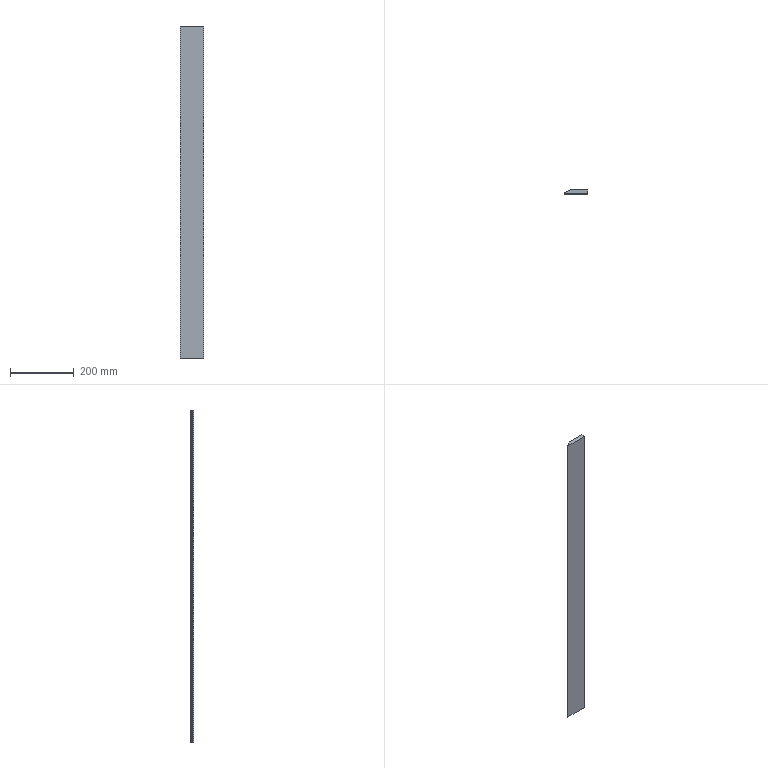Part | SolidWorks | features FlatPattern 1, SMBaseFlange 1, SheetMetal 1 | 1 solid | 7 faces | box 75 x 12 x 1040 mm | volume 832000 mm3 | plane 7
STEP:
#1=CARTESIAN_POINT('',(55.,0.,0.));
#2=VERTEX_POINT('',#1);
#3=CARTESIAN_POINT('',(55.,12.,0.));
#4=VERTEX_POINT('',#3);
#5=CARTESIAN_POINT('',(55.,12.,0.));
#6=DIRECTION('',(0.,1.,0.));
#7=VECTOR('',#6,1000.);
#8=LINE('',#5,#7);
#9=EDGE_CURVE('',#2,#4,#8,.T.);
#10=ORIENTED_EDGE('',*,*,#9,.F.);
#11=CARTESIAN_POINT('',(55.,0.,-1040.));
#12=VERTEX_POINT('',#11);
#13=CARTESIAN_POINT('',(55.,0.,-1040.));
#14=DIRECTION('',(0.,0.,1.));
#15=VECTOR('',#14,1000.);
#16=LINE('',#13,#15);
#17=EDGE_CURVE('',#12,#2,#16,.T.);
#18=ORIENTED_EDGE('',*,*,#17,.F.);
#19=CARTESIAN_POINT('',(55.,12.,-1040.));
#20=VERTEX_POINT('',#19);
#21=CARTESIAN_POINT('',(55.,12.,-1040.));
#22=DIRECTION('',(0.,1.,0.));
#23=VECTOR('',#22,1000.);
#24=LINE('',#21,#23);
#25=EDGE_CURVE('',#12,#20,#24,.T.);
#26=ORIENTED_EDGE('',*,*,#25,.T.);
#27=CARTESIAN_POINT('',(55.,12.,-1040.));
#28=DIRECTION('',(0.,0.,1.));
#29=VECTOR('',#28,1000.);
#30=LINE('',#27,#29);
#31=EDGE_CURVE('',#20,#4,#30,.T.);
#32=ORIENTED_EDGE('',*,*,#31,.T.);
#33=EDGE_LOOP('',(#10,#18,#26,#32));
#34=FACE_OUTER_BOUND('',#33,.T.);
#35=CARTESIAN_POINT('',(55.,12.,-1040.));
#36=DIRECTION('',(1.,0.,0.));
#37=DIRECTION('',(0.,1.,0.));
#38=AXIS2_PLACEMENT_3D('',#35,#36,#37);
#39=PLANE('',#38);
#40=ADVANCED_FACE('',(#34),#39,.T.);
#41=CARTESIAN_POINT('',(-20.,0.,0.));
#42=VERTEX_POINT('',#41);
#43=CARTESIAN_POINT('',(55.,0.,0.));
#44=DIRECTION('',(1.,0.,0.));
#45=VECTOR('',#44,1000.);
#46=LINE('',#43,#45);
#47=EDGE_CURVE('',#42,#2,#46,.T.);
#48=ORIENTED_EDGE('',*,*,#47,.F.);
#49=CARTESIAN_POINT('',(-20.,0.,-1040.));
#50=VERTEX_POINT('',#49);
#51=CARTESIAN_POINT('',(-20.,0.,-1040.));
#52=DIRECTION('',(0.,0.,1.));
#53=VECTOR('',#52,1000.);
#54=LINE('',#51,#53);
#55=EDGE_CURVE('',#50,#42,#54,.T.);
#56=ORIENTED_EDGE('',*,*,#55,.F.);
#57=CARTESIAN_POINT('',(55.,0.,-1040.));
#58=DIRECTION('',(1.,0.,0.));
#59=VECTOR('',#58,1000.);
#60=LINE('',#57,#59);
#61=EDGE_CURVE('',#50,#12,#60,.T.);
#62=ORIENTED_EDGE('',*,*,#61,.T.);
#63=ORIENTED_EDGE('',*,*,#17,.T.);
#64=EDGE_LOOP('',(#48,#56,#62,#63));
#65=FACE_OUTER_BOUND('',#64,.T.);
#66=CARTESIAN_POINT('',(55.,0.,-1040.));
#67=DIRECTION('',(0.,-1.,0.));
#68=DIRECTION('',(1.,0.,0.));
#69=AXIS2_PLACEMENT_3D('',#66,#67,#68);
#70=PLANE('',#69);
#71=ADVANCED_FACE('',(#65),#70,.T.);
#72=CARTESIAN_POINT('',(-20.,2.,0.));
#73=VERTEX_POINT('',#72);
#74=CARTESIAN_POINT('',(-20.,0.,0.));
#75=DIRECTION('',(0.,-1.,0.));
#76=VECTOR('',#75,1000.);
#77=LINE('',#74,#76);
#78=EDGE_CURVE('',#73,#42,#77,.T.);
#79=ORIENTED_EDGE('',*,*,#78,.F.);
#80=CARTESIAN_POINT('',(-20.,2.,-1040.));
#81=VERTEX_POINT('',#80);
#82=CARTESIAN_POINT('',(-20.,2.,-1040.));
#83=DIRECTION('',(0.,0.,1.));
#84=VECTOR('',#83,1000.);
#85=LINE('',#82,#84);
#86=EDGE_CURVE('',#81,#73,#85,.T.);
#87=ORIENTED_EDGE('',*,*,#86,.F.);
#88=CARTESIAN_POINT('',(-20.,0.,-1040.));
#89=DIRECTION('',(0.,-1.,0.));
#90=VECTOR('',#89,1000.);
#91=LINE('',#88,#90);
#92=EDGE_CURVE('',#81,#50,#91,.T.);
#93=ORIENTED_EDGE('',*,*,#92,.T.);
#94=ORIENTED_EDGE('',*,*,#55,.T.);
#95=EDGE_LOOP('',(#79,#87,#93,#94));
#96=FACE_OUTER_BOUND('',#95,.T.);
#97=CARTESIAN_POINT('',(-20.,0.,-1040.));
#98=DIRECTION('',(-1.,0.,0.));
#99=DIRECTION('',(0.,-1.,0.));
#100=AXIS2_PLACEMENT_3D('',#97,#98,#99);
#101=PLANE('',#100);
#102=ADVANCED_FACE('',(#96),#101,.T.);
#103=CARTESIAN_POINT('',(0.,12.,0.));
#104=VERTEX_POINT('',#103);
#105=CARTESIAN_POINT('',(-20.,2.,0.));
#106=DIRECTION('',(-0.8944,-0.4472,0.));
#107=VECTOR('',#106,1000.);
#108=LINE('',#105,#107);
#109=EDGE_CURVE('',#104,#73,#108,.T.);
#110=ORIENTED_EDGE('',*,*,#109,.F.);
#111=CARTESIAN_POINT('',(0.,12.,-1040.));
#112=VERTEX_POINT('',#111);
#113=CARTESIAN_POINT('',(0.,12.,-1040.));
#114=DIRECTION('',(0.,0.,1.));
#115=VECTOR('',#114,1000.);
#116=LINE('',#113,#115);
#117=EDGE_CURVE('',#112,#104,#116,.T.);
#118=ORIENTED_EDGE('',*,*,#117,.F.);
#119=CARTESIAN_POINT('',(-20.,2.,-1040.));
#120=DIRECTION('',(-0.8944,-0.4472,0.));
#121=VECTOR('',#120,1000.);
#122=LINE('',#119,#121);
#123=EDGE_CURVE('',#112,#81,#122,.T.);
#124=ORIENTED_EDGE('',*,*,#123,.T.);
#125=ORIENTED_EDGE('',*,*,#86,.T.);
#126=EDGE_LOOP('',(#110,#118,#124,#125));
#127=FACE_OUTER_BOUND('',#126,.T.);
#128=CARTESIAN_POINT('',(-20.,2.,-1040.));
#129=DIRECTION('',(-0.4472,0.8944,0.));
#130=DIRECTION('',(-0.8944,-0.4472,0.));
#131=AXIS2_PLACEMENT_3D('',#128,#129,#130);
#132=PLANE('',#131);
#133=ADVANCED_FACE('',(#127),#132,.T.);
#134=CARTESIAN_POINT('',(0.,12.,0.));
#135=DIRECTION('',(-1.,0.,0.));
#136=VECTOR('',#135,1000.);
#137=LINE('',#134,#136);
#138=EDGE_CURVE('',#4,#104,#137,.T.);
#139=ORIENTED_EDGE('',*,*,#138,.F.);
#140=ORIENTED_EDGE('',*,*,#31,.F.);
#141=CARTESIAN_POINT('',(0.,12.,-1040.));
#142=DIRECTION('',(-1.,0.,0.));
#143=VECTOR('',#142,1000.);
#144=LINE('',#141,#143);
#145=EDGE_CURVE('',#20,#112,#144,.T.);
#146=ORIENTED_EDGE('',*,*,#145,.T.);
#147=ORIENTED_EDGE('',*,*,#117,.T.);
#148=EDGE_LOOP('',(#139,#140,#146,#147));
#149=FACE_OUTER_BOUND('',#148,.T.);
#150=CARTESIAN_POINT('',(0.,12.,-1040.));
#151=DIRECTION('',(0.,1.,0.));
#152=DIRECTION('',(0.,0.,1.));
#153=AXIS2_PLACEMENT_3D('',#150,#151,#152);
#154=PLANE('',#153);
#155=ADVANCED_FACE('',(#149),#154,.T.);
#156=ORIENTED_EDGE('',*,*,#25,.F.);
#157=ORIENTED_EDGE('',*,*,#61,.F.);
#158=ORIENTED_EDGE('',*,*,#92,.F.);
#159=ORIENTED_EDGE('',*,*,#123,.F.);
#160=ORIENTED_EDGE('',*,*,#145,.F.);
#161=EDGE_LOOP('',(#156,#157,#158,#159,#160));
#162=FACE_OUTER_BOUND('',#161,.T.);
#163=CARTESIAN_POINT('',(0.,0.,-1040.));
#164=DIRECTION('',(0.,0.,-1.));
#165=DIRECTION('',(-1.,0.,0.));
#166=AXIS2_PLACEMENT_3D('',#163,#164,#165);
#167=PLANE('',#166);
#168=ADVANCED_FACE('',(#162),#167,.T.);
#169=ORIENTED_EDGE('',*,*,#9,.T.);
#170=ORIENTED_EDGE('',*,*,#138,.T.);
#171=ORIENTED_EDGE('',*,*,#109,.T.);
#172=ORIENTED_EDGE('',*,*,#78,.T.);
#173=ORIENTED_EDGE('',*,*,#47,.T.);
#174=EDGE_LOOP('',(#169,#170,#171,#172,#173));
#175=FACE_OUTER_BOUND('',#174,.T.);
#176=CARTESIAN_POINT('',(0.,0.,0.));
#177=DIRECTION('',(0.,0.,-1.));
#178=DIRECTION('',(-1.,0.,0.));
#179=AXIS2_PLACEMENT_3D('',#176,#177,#178);
#180=PLANE('',#179);
#181=ADVANCED_FACE('',(#175),#180,.F.);
#182=CLOSED_SHELL('',(#40,#71,#102,#133,#155,#168,#181));
#183=MANIFOLD_SOLID_BREP('',#182);
#184=CARTESIAN_POINT('',(0.,0.,0.));
#185=DIRECTION('',(0.,0.,1.));
#186=DIRECTION('',(1.,0.,0.));
#187=AXIS2_PLACEMENT_3D('',#184,#185,#186);
#188=(LENGTH_UNIT()NAMED_UNIT(*)SI_UNIT(.MILLI.,.METRE.));
#189=UNCERTAINTY_MEASURE_WITH_UNIT(LENGTH_MEASURE(0.00001),#188,'','');
#190=(NAMED_UNIT(*)PLANE_ANGLE_UNIT()SI_UNIT($,.RADIAN.));
#191=(NAMED_UNIT(*)SI_UNIT($,.STERADIAN.)SOLID_ANGLE_UNIT());
#192=(GEOMETRIC_REPRESENTATION_CONTEXT(3)GLOBAL_UNCERTAINTY_ASSIGNED_CONTEXT((#189))GLOBAL_UNIT_ASSIGNED_CONTEXT((#188,#190,#191))REPRESENTATION_CONTEXT('',''));
#193=ADVANCED_BREP_SHAPE_REPRESENTATION('',(#183,#187),#192);